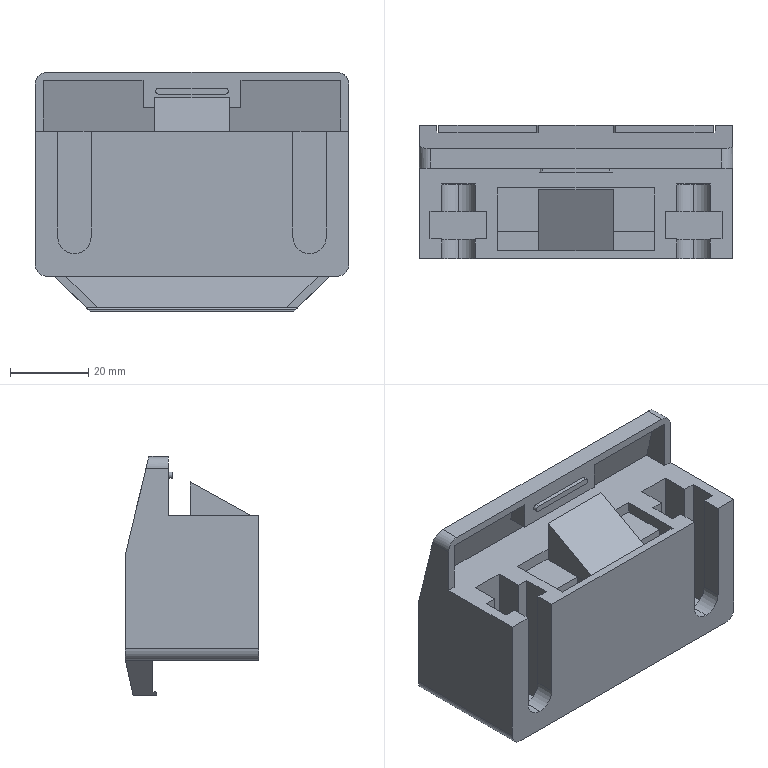Part | NX | features BREP 1 | 1 solid | 115 faces | box 80 x 34 x 61 mm | volume 88371 mm3 | plane 94 | cylinder 21 | commonest cylinder face diameters 8.5 x8 6 x4 1.5 x2 15 x2 16 x2 1 x1